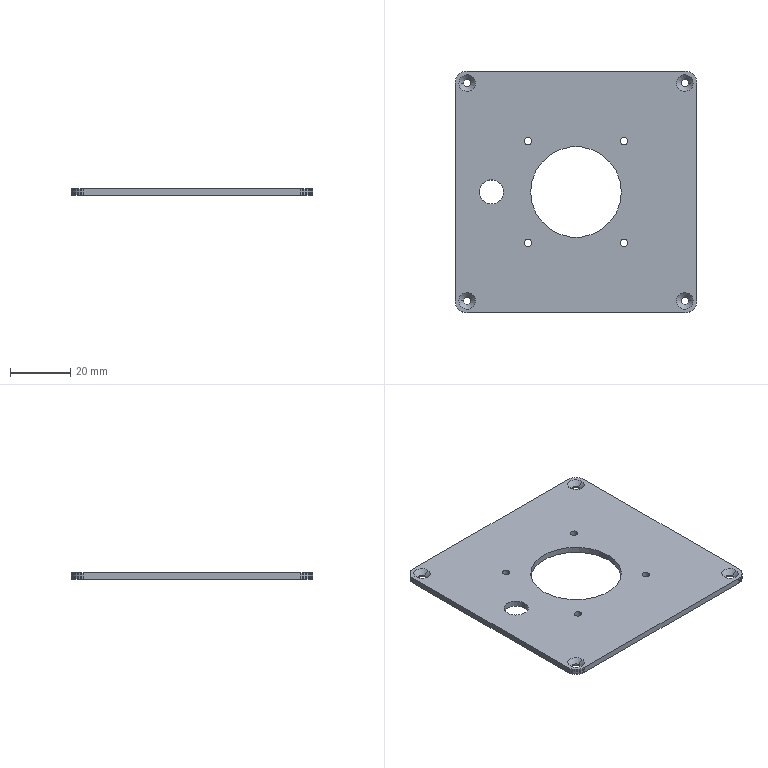Part | SolidWorks | features ICE 4, Chamfer 1, Extrusion 1, MoveFace 1 | 1 solid | 82 faces | box 80 x 80 x 2 mm | volume 11130 mm3 | plane 54 | cylinder 20 | cone 8 | commonest cylinder face diameters 2.5 x16 8 x2 30 x2